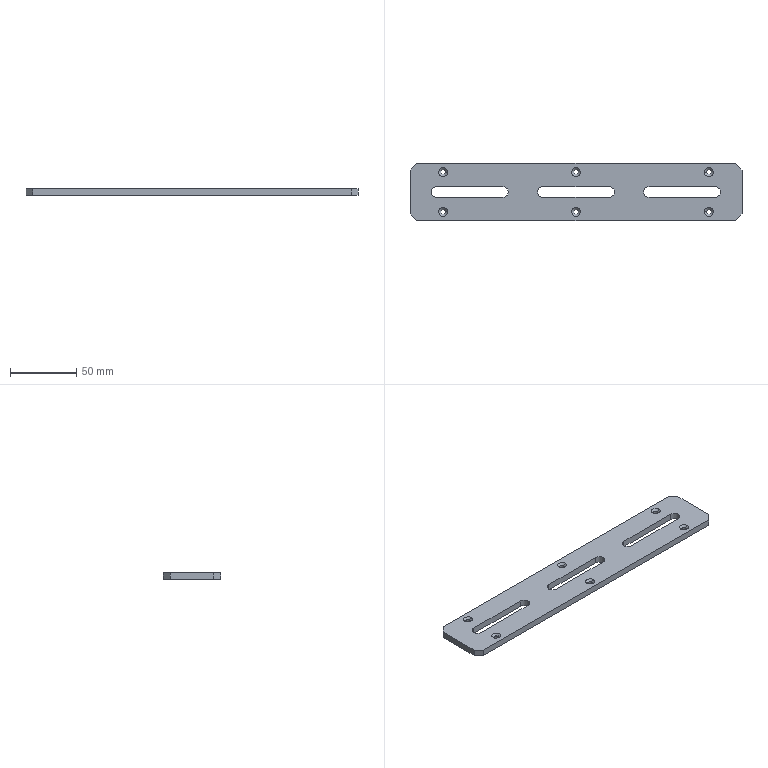Part | STEP file | B02 | 1 solid | 49 faces | box 250 x 43 x 5 mm | volume 46334 mm3 | cylinder 21 | plane 16 | cone 12 | commonest cylinder face diameters 3.6 x12 8 x9